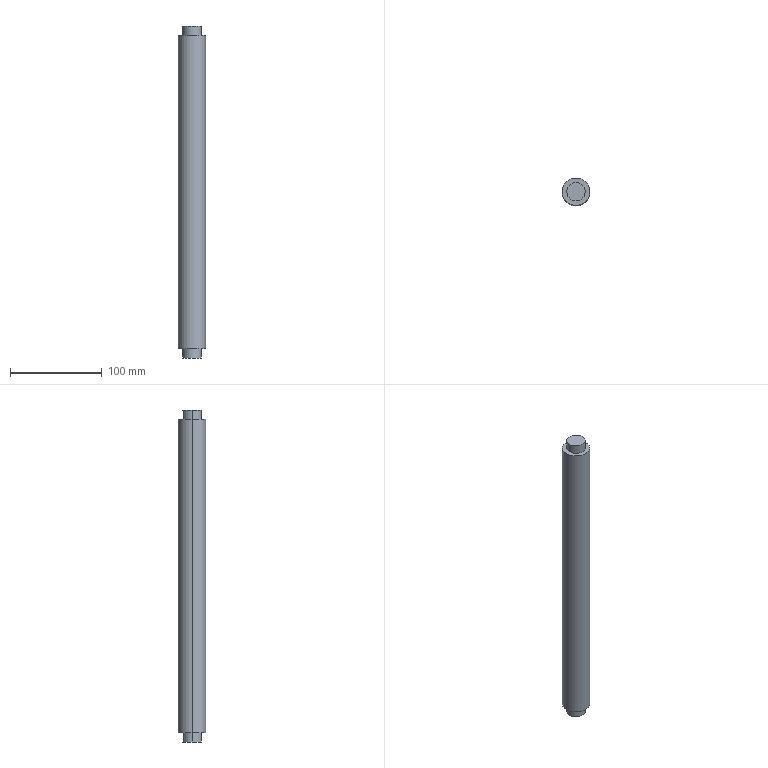Part | SolidWorks | features Extrusion 1, ICE 1, MirrorPattern 1 | 1 solid | 10 faces | box 30 x 30 x 361 mm | volume 247322 mm3 | cylinder 6 | plane 4 | commonest cylinder face diameters 20 x4 30 x2
STEP:
#1=CARTESIAN_POINT('',(10.,0.,-180.5));
#2=VERTEX_POINT('',#1);
#3=CARTESIAN_POINT('',(-10.,0.,-180.5));
#4=VERTEX_POINT('',#3);
#5=CARTESIAN_POINT('',(0.,0.,-180.5));
#6=DIRECTION('',(0.,0.,1.));
#7=DIRECTION('',(1.,0.,0.));
#8=AXIS2_PLACEMENT_3D('',#5,#6,#7);
#9=CIRCLE('',#8,10.);
#10=EDGE_CURVE('',#2,#4,#9,.T.);
#11=ORIENTED_EDGE('',*,*,#10,.T.);
#12=CARTESIAN_POINT('',(-10.,0.,-170.5));
#13=VERTEX_POINT('',#12);
#14=CARTESIAN_POINT('',(-10.,0.,-180.5));
#15=DIRECTION('',(0.,0.,1.));
#16=VECTOR('',#15,1000.);
#17=LINE('',#14,#16);
#18=EDGE_CURVE('',#4,#13,#17,.T.);
#19=ORIENTED_EDGE('',*,*,#18,.T.);
#20=CARTESIAN_POINT('',(10.,0.,-170.5));
#21=VERTEX_POINT('',#20);
#22=CARTESIAN_POINT('',(0.,0.,-170.5));
#23=DIRECTION('',(0.,0.,1.));
#24=DIRECTION('',(1.,0.,0.));
#25=AXIS2_PLACEMENT_3D('',#22,#23,#24);
#26=CIRCLE('',#25,10.);
#27=EDGE_CURVE('',#21,#13,#26,.T.);
#28=ORIENTED_EDGE('',*,*,#27,.F.);
#29=CARTESIAN_POINT('',(10.,0.,-180.5));
#30=DIRECTION('',(0.,0.,1.));
#31=VECTOR('',#30,1000.);
#32=LINE('',#29,#31);
#33=EDGE_CURVE('',#2,#21,#32,.T.);
#34=ORIENTED_EDGE('',*,*,#33,.F.);
#35=EDGE_LOOP('',(#11,#19,#28,#34));
#36=FACE_OUTER_BOUND('',#35,.T.);
#37=CARTESIAN_POINT('',(0.,0.,-180.5));
#38=DIRECTION('',(0.,0.,1.));
#39=DIRECTION('',(1.,0.,0.));
#40=AXIS2_PLACEMENT_3D('',#37,#38,#39);
#41=CYLINDRICAL_SURFACE('',#40,10.);
#42=ADVANCED_FACE('',(#36),#41,.T.);
#43=CARTESIAN_POINT('',(10.,0.,180.5));
#44=VERTEX_POINT('',#43);
#45=CARTESIAN_POINT('',(-10.,0.,180.5));
#46=VERTEX_POINT('',#45);
#47=CARTESIAN_POINT('',(0.,0.,180.5));
#48=DIRECTION('',(0.,0.,1.));
#49=DIRECTION('',(1.,0.,0.));
#50=AXIS2_PLACEMENT_3D('',#47,#48,#49);
#51=CIRCLE('',#50,10.);
#52=EDGE_CURVE('',#44,#46,#51,.T.);
#53=ORIENTED_EDGE('',*,*,#52,.F.);
#54=CARTESIAN_POINT('',(10.,0.,170.5));
#55=VERTEX_POINT('',#54);
#56=CARTESIAN_POINT('',(10.,0.,180.5));
#57=DIRECTION('',(0.,0.,-1.));
#58=VECTOR('',#57,1000.);
#59=LINE('',#56,#58);
#60=EDGE_CURVE('',#44,#55,#59,.T.);
#61=ORIENTED_EDGE('',*,*,#60,.T.);
#62=CARTESIAN_POINT('',(-10.,0.,170.5));
#63=VERTEX_POINT('',#62);
#64=CARTESIAN_POINT('',(0.,0.,170.5));
#65=DIRECTION('',(0.,0.,1.));
#66=DIRECTION('',(1.,0.,0.));
#67=AXIS2_PLACEMENT_3D('',#64,#65,#66);
#68=CIRCLE('',#67,10.);
#69=EDGE_CURVE('',#55,#63,#68,.T.);
#70=ORIENTED_EDGE('',*,*,#69,.T.);
#71=CARTESIAN_POINT('',(-10.,0.,180.5));
#72=DIRECTION('',(0.,0.,-1.));
#73=VECTOR('',#72,1000.);
#74=LINE('',#71,#73);
#75=EDGE_CURVE('',#46,#63,#74,.T.);
#76=ORIENTED_EDGE('',*,*,#75,.F.);
#77=EDGE_LOOP('',(#53,#61,#70,#76));
#78=FACE_OUTER_BOUND('',#77,.T.);
#79=CARTESIAN_POINT('',(0.,0.,180.5));
#80=DIRECTION('',(0.,0.,-1.));
#81=DIRECTION('',(-1.,0.,0.));
#82=AXIS2_PLACEMENT_3D('',#79,#80,#81);
#83=CYLINDRICAL_SURFACE('',#82,10.);
#84=ADVANCED_FACE('',(#78),#83,.T.);
#85=CARTESIAN_POINT('',(15.,0.,170.5));
#86=VERTEX_POINT('',#85);
#87=CARTESIAN_POINT('',(-15.,0.,170.5));
#88=VERTEX_POINT('',#87);
#89=CARTESIAN_POINT('',(0.,0.,170.5));
#90=DIRECTION('',(0.,0.,1.));
#91=DIRECTION('',(1.,0.,0.));
#92=AXIS2_PLACEMENT_3D('',#89,#90,#91);
#93=CIRCLE('',#92,15.);
#94=EDGE_CURVE('',#86,#88,#93,.T.);
#95=ORIENTED_EDGE('',*,*,#94,.F.);
#96=CARTESIAN_POINT('',(15.,0.,-170.5));
#97=VERTEX_POINT('',#96);
#98=CARTESIAN_POINT('',(15.,0.,170.5));
#99=DIRECTION('',(0.,0.,-1.));
#100=VECTOR('',#99,1000.);
#101=LINE('',#98,#100);
#102=EDGE_CURVE('',#86,#97,#101,.T.);
#103=ORIENTED_EDGE('',*,*,#102,.T.);
#104=CARTESIAN_POINT('',(-15.,0.,-170.5));
#105=VERTEX_POINT('',#104);
#106=CARTESIAN_POINT('',(0.,0.,-170.5));
#107=DIRECTION('',(0.,0.,1.));
#108=DIRECTION('',(1.,0.,0.));
#109=AXIS2_PLACEMENT_3D('',#106,#107,#108);
#110=CIRCLE('',#109,15.);
#111=EDGE_CURVE('',#97,#105,#110,.T.);
#112=ORIENTED_EDGE('',*,*,#111,.T.);
#113=CARTESIAN_POINT('',(-15.,0.,170.5));
#114=DIRECTION('',(0.,0.,-1.));
#115=VECTOR('',#114,1000.);
#116=LINE('',#113,#115);
#117=EDGE_CURVE('',#88,#105,#116,.T.);
#118=ORIENTED_EDGE('',*,*,#117,.F.);
#119=EDGE_LOOP('',(#95,#103,#112,#118));
#120=FACE_OUTER_BOUND('',#119,.T.);
#121=CARTESIAN_POINT('',(0.,0.,170.5));
#122=DIRECTION('',(0.,0.,-1.));
#123=DIRECTION('',(-1.,0.,0.));
#124=AXIS2_PLACEMENT_3D('',#121,#122,#123);
#125=CYLINDRICAL_SURFACE('',#124,15.);
#126=ADVANCED_FACE('',(#120),#125,.T.);
#127=ORIENTED_EDGE('',*,*,#102,.F.);
#128=CARTESIAN_POINT('',(0.,0.,170.5));
#129=DIRECTION('',(0.,0.,1.));
#130=DIRECTION('',(1.,0.,0.));
#131=AXIS2_PLACEMENT_3D('',#128,#129,#130);
#132=CIRCLE('',#131,15.);
#133=EDGE_CURVE('',#88,#86,#132,.T.);
#134=ORIENTED_EDGE('',*,*,#133,.F.);
#135=ORIENTED_EDGE('',*,*,#117,.T.);
#136=CARTESIAN_POINT('',(0.,0.,-170.5));
#137=DIRECTION('',(0.,0.,1.));
#138=DIRECTION('',(1.,0.,0.));
#139=AXIS2_PLACEMENT_3D('',#136,#137,#138);
#140=CIRCLE('',#139,15.);
#141=EDGE_CURVE('',#105,#97,#140,.T.);
#142=ORIENTED_EDGE('',*,*,#141,.T.);
#143=EDGE_LOOP('',(#127,#134,#135,#142));
#144=FACE_OUTER_BOUND('',#143,.T.);
#145=CARTESIAN_POINT('',(0.,0.,170.5));
#146=DIRECTION('',(0.,0.,-1.));
#147=DIRECTION('',(-1.,0.,0.));
#148=AXIS2_PLACEMENT_3D('',#145,#146,#147);
#149=CYLINDRICAL_SURFACE('',#148,15.);
#150=ADVANCED_FACE('',(#144),#149,.T.);
#151=CARTESIAN_POINT('',(0.,0.,170.5));
#152=DIRECTION('',(0.,0.,1.));
#153=DIRECTION('',(1.,0.,0.));
#154=AXIS2_PLACEMENT_3D('',#151,#152,#153);
#155=CIRCLE('',#154,10.);
#156=EDGE_CURVE('',#63,#55,#155,.T.);
#157=ORIENTED_EDGE('',*,*,#156,.F.);
#158=ORIENTED_EDGE('',*,*,#69,.F.);
#159=EDGE_LOOP('',(#157,#158));
#160=FACE_BOUND('',#159,.T.);
#161=ORIENTED_EDGE('',*,*,#133,.T.);
#162=ORIENTED_EDGE('',*,*,#94,.T.);
#163=EDGE_LOOP('',(#161,#162));
#164=FACE_OUTER_BOUND('',#163,.T.);
#165=CARTESIAN_POINT('',(0.,0.,170.5));
#166=DIRECTION('',(0.,0.,1.));
#167=DIRECTION('',(1.,0.,0.));
#168=AXIS2_PLACEMENT_3D('',#165,#166,#167);
#169=PLANE('',#168);
#170=ADVANCED_FACE('',(#160,#164),#169,.T.);
#171=ORIENTED_EDGE('',*,*,#27,.T.);
#172=CARTESIAN_POINT('',(0.,0.,-170.5));
#173=DIRECTION('',(0.,0.,1.));
#174=DIRECTION('',(1.,0.,0.));
#175=AXIS2_PLACEMENT_3D('',#172,#173,#174);
#176=CIRCLE('',#175,10.);
#177=EDGE_CURVE('',#13,#21,#176,.T.);
#178=ORIENTED_EDGE('',*,*,#177,.T.);
#179=EDGE_LOOP('',(#171,#178));
#180=FACE_BOUND('',#179,.T.);
#181=ORIENTED_EDGE('',*,*,#141,.F.);
#182=ORIENTED_EDGE('',*,*,#111,.F.);
#183=EDGE_LOOP('',(#181,#182));
#184=FACE_OUTER_BOUND('',#183,.T.);
#185=CARTESIAN_POINT('',(0.,0.,-170.5));
#186=DIRECTION('',(0.,0.,1.));
#187=DIRECTION('',(1.,0.,0.));
#188=AXIS2_PLACEMENT_3D('',#185,#186,#187);
#189=PLANE('',#188);
#190=ADVANCED_FACE('',(#180,#184),#189,.F.);
#191=ORIENTED_EDGE('',*,*,#60,.F.);
#192=CARTESIAN_POINT('',(0.,0.,180.5));
#193=DIRECTION('',(0.,0.,1.));
#194=DIRECTION('',(1.,0.,0.));
#195=AXIS2_PLACEMENT_3D('',#192,#193,#194);
#196=CIRCLE('',#195,10.);
#197=EDGE_CURVE('',#46,#44,#196,.T.);
#198=ORIENTED_EDGE('',*,*,#197,.F.);
#199=ORIENTED_EDGE('',*,*,#75,.T.);
#200=ORIENTED_EDGE('',*,*,#156,.T.);
#201=EDGE_LOOP('',(#191,#198,#199,#200));
#202=FACE_OUTER_BOUND('',#201,.T.);
#203=CARTESIAN_POINT('',(0.,0.,180.5));
#204=DIRECTION('',(0.,0.,-1.));
#205=DIRECTION('',(-1.,0.,0.));
#206=AXIS2_PLACEMENT_3D('',#203,#204,#205);
#207=CYLINDRICAL_SURFACE('',#206,10.);
#208=ADVANCED_FACE('',(#202),#207,.T.);
#209=ORIENTED_EDGE('',*,*,#197,.T.);
#210=ORIENTED_EDGE('',*,*,#52,.T.);
#211=EDGE_LOOP('',(#209,#210));
#212=FACE_OUTER_BOUND('',#211,.T.);
#213=CARTESIAN_POINT('',(0.,0.,180.5));
#214=DIRECTION('',(0.,0.,1.));
#215=DIRECTION('',(1.,0.,0.));
#216=AXIS2_PLACEMENT_3D('',#213,#214,#215);
#217=PLANE('',#216);
#218=ADVANCED_FACE('',(#212),#217,.T.);
#219=ORIENTED_EDGE('',*,*,#18,.F.);
#220=CARTESIAN_POINT('',(0.,0.,-180.5));
#221=DIRECTION('',(0.,0.,1.));
#222=DIRECTION('',(1.,0.,0.));
#223=AXIS2_PLACEMENT_3D('',#220,#221,#222);
#224=CIRCLE('',#223,10.);
#225=EDGE_CURVE('',#4,#2,#224,.T.);
#226=ORIENTED_EDGE('',*,*,#225,.T.);
#227=ORIENTED_EDGE('',*,*,#33,.T.);
#228=ORIENTED_EDGE('',*,*,#177,.F.);
#229=EDGE_LOOP('',(#219,#226,#227,#228));
#230=FACE_OUTER_BOUND('',#229,.T.);
#231=CARTESIAN_POINT('',(0.,0.,-180.5));
#232=DIRECTION('',(0.,0.,1.));
#233=DIRECTION('',(1.,0.,0.));
#234=AXIS2_PLACEMENT_3D('',#231,#232,#233);
#235=CYLINDRICAL_SURFACE('',#234,10.);
#236=ADVANCED_FACE('',(#230),#235,.T.);
#237=ORIENTED_EDGE('',*,*,#10,.F.);
#238=ORIENTED_EDGE('',*,*,#225,.F.);
#239=EDGE_LOOP('',(#237,#238));
#240=FACE_OUTER_BOUND('',#239,.T.);
#241=CARTESIAN_POINT('',(0.,0.,-180.5));
#242=DIRECTION('',(0.,0.,-1.));
#243=DIRECTION('',(1.,0.,0.));
#244=AXIS2_PLACEMENT_3D('',#241,#242,#243);
#245=PLANE('',#244);
#246=ADVANCED_FACE('',(#240),#245,.T.);
#247=CLOSED_SHELL('',(#42,#84,#126,#150,#170,#190,#208,#218,#236,#246));
#248=MANIFOLD_SOLID_BREP('',#247);
#249=CARTESIAN_POINT('',(0.,0.,0.));
#250=DIRECTION('',(0.,0.,1.));
#251=DIRECTION('',(1.,0.,0.));
#252=AXIS2_PLACEMENT_3D('',#249,#250,#251);
#253=(LENGTH_UNIT()NAMED_UNIT(*)SI_UNIT(.MILLI.,.METRE.));
#254=UNCERTAINTY_MEASURE_WITH_UNIT(LENGTH_MEASURE(0.00001),#253,'','');
#255=(NAMED_UNIT(*)PLANE_ANGLE_UNIT()SI_UNIT($,.RADIAN.));
#256=(NAMED_UNIT(*)SI_UNIT($,.STERADIAN.)SOLID_ANGLE_UNIT());
#257=(GEOMETRIC_REPRESENTATION_CONTEXT(3)GLOBAL_UNCERTAINTY_ASSIGNED_CONTEXT((#254))GLOBAL_UNIT_ASSIGNED_CONTEXT((#253,#255,#256))REPRESENTATION_CONTEXT('',''));
#258=ADVANCED_BREP_SHAPE_REPRESENTATION('',(#248,#252),#257);